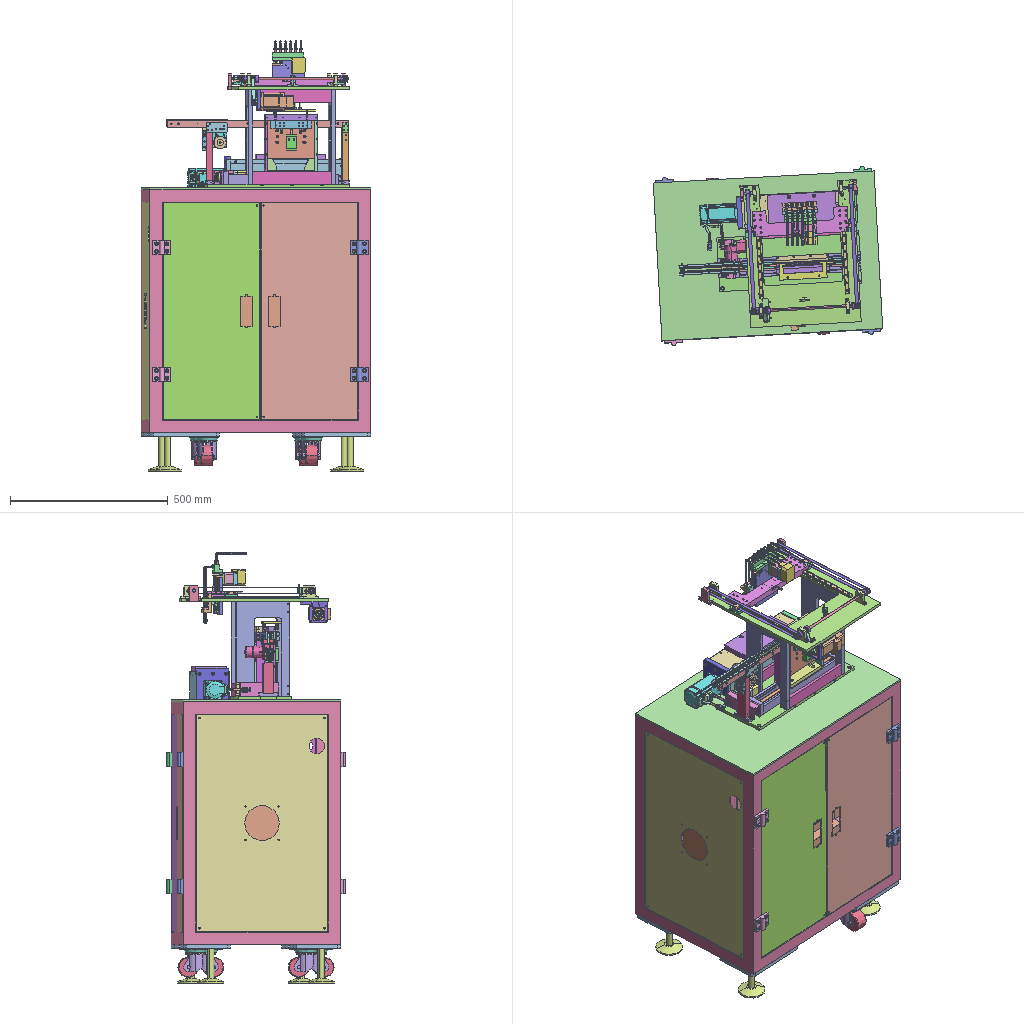Assembly | SolidWorks | 162 different items | 352 placed | box 726 x 565 x 1363 mm
Parts list (item | name | quantity | parent item | size | volume | features):
1 | (subassembly) | x2 | in 11 | 59.5 x 34.5 x 13 mm | 14643 mm3 | -
2 | (subassembly) | x1 | - | 120 x 12 x 21.25 mm | 21373 mm3 | -
3 | (subassembly) | x1 | - | 166.8 x 105 x 498.5 mm | 1079493 mm3 | -
4 | (subassembly) | x4 | in 6 | 102.5 x 91.977 x 71 mm | 201303 mm3 | -
5 | (subassembly) | x1 | - | 700 x 892 x 532 mm | 21154344 mm3 | -
6 | (subassembly) | x4 | in 5, 7 | 222 x 156.5 x 180 mm | 695134 mm3 | -
7 | (subassembly) | x2 | in 5 | 222 x 156.5 x 180 mm | 695134 mm3 | -
8 | (subassembly) | x1 | in 10 | 41 x 53 x 93.5 mm | 138509 mm3 | -
9 | (subassembly) | x1 | - | 41.5 x 52 x 94 mm | 136281 mm3 | -
10 | (subassembly) | x1 | in 11 | 131.635 x 44 x 404.935 mm | 615573 mm3 | -
11 | (subassembly) | x1 | - | 575.911 x 235.705 x 185.668 mm | 2678930 mm3 | -
12 | - | x1 | in 5 | 560 x 600 x 263 mm | 1044894 mm3 | features BaseBody 1
13 | - | x1 | - | 34 x 31 x 5 mm | 2038 mm3 | features BaseBody 1
14 | - | x2 | - | 5 x 5 x 50 mm | 981.136 mm3 | features BaseBody 1
15 | - | x1 | - | 350 x 8 x 8 mm | 17587 mm3 | features BaseBody 1
16 | - | x2 | - | 8 x 8 x 45 mm | 2262 mm3 | features BaseBody 1
17 | - | x6 | - | 10 x 10 x 77 mm | 1624 mm3 | features BaseBody 1
18 | - | x2 | in 2 | 5.001 x 5.001 x 5.2 mm | 8.924 mm3 | features BaseBody 1
19 | - | x2 | - | 17 x 23.4 x 6.7 mm | 1902 mm3 | features BaseBody 1
20 | - | x6 | - | 15 x 15 x 5 mm | 961.952 mm3 | features BaseBody 1
21 | - | x3 | - | 40 x 250 x 10 mm | 99178 mm3 | features BaseBody 1
22 | - | x1 | in 11 | 150 x 120 x 8 mm | 141574 mm3 | features BaseBody 1
23 | - | x1 | in 5 | 620 x 420 x 15 mm | 428208 mm3 | features BaseBody 1
24 | - | x1 | in 11 | 150 x 25 x 8 mm | 29604 mm3 | features BaseBody 1
25 | - | x2 | in 11 | 538 x 10 x 6 mm | 32064 mm3 | features BaseBody 1
26 | - | x1 | in 11 | 169.5 x 60 x 8 mm | 71017 mm3 | features BaseBody 1
27 | - | x1 | in 11 | 169.5 x 60 x 8 mm | 70941 mm3 | features BaseBody 1
28 | - | x2 | in 11 | 30 x 50 x 9 mm | 9481 mm3 | features BaseBody 1
29 | - | x1 | in 11 | 150 x 60 x 12 mm | 103321 mm3 | features BaseBody 1
30 | - | x1 | in 11 | 575 x 20 x 6 mm | 67891 mm3 | features BaseBody 1
31 | - | x1 | in 11 | 575 x 20 x 6 mm | 67891 mm3 | features BaseBody 1
32 | - | x2 | in 11 | 5 x 5 x 9 mm | 165.64 mm3 | features BaseBody 1
33 | - | x2 | in 2 | 3 x 3 x 16 mm | 111.003 mm3 | features BaseBody 1
34 | - | x4 | in 4 | 42 x 13 x 13 mm | 5217 mm3 | features BaseBody 1
35 | - | x2 | in 11 | 30 x 65 x 3 mm | 5483 mm3 | features BaseBody 1
36 | - | x1 | in 11 | 35 x 27 x 14.5 mm | 4375 mm3 | features BaseBody 1
37 | - | x1 | in 11 | 37 x 37 x 79.2 mm | 56499 mm3 | features BaseBody 1
38 | - | x6 | - | 10 x 10 x 13.5 mm | 457.625 mm3 | features BaseBody 1
39 | - | x1 | - | 110 x 34 x 10 mm | 36400 mm3 | features BaseBody 1
40 | - | x1 | - | 100 x 26 x 25 mm | 48829 mm3 | features BaseBody 1
41 | - | x6 | - | 8.007 x 8.002 x 20 mm | 45.848 mm3 | features BaseBody 1
42 | - | x2 | in 1 | 43 x 24 x 13 mm | 9011 mm3 | features BaseBody 1
43 | - | x2 | in 1 | 12 x 46 x 5 mm | 2467 mm3 | features BaseBody 1
44 | - | x1 | - | 16 x 11 x 16 mm | 1494 mm3 | features BaseBody 1
45 | - | x4 | in 4 | 66 x 58.3 x 58 mm | 18491 mm3 | features BaseBody 1
46 | - | x2 | - | 27 x 10 x 33.9 mm | 6982 mm3 | features BaseBody 1
47 | - | x1 | in 8 | 41 x 42.5 x 11.5 mm | 19594 mm3 | features BaseBody 1
48 | - | x1 | in 10 | 27.5 x 96.5 x 6 mm | 1654 mm3 | features BaseBody 1
49 | - | x1 | in 10 | 42.935 x 28.935 x 122.935 mm | 4950 mm3 | features BaseBody 1
50 | - | x1 | in 10 | 30 x 30 x 10.4 mm | 5208 mm3 | features BaseBody 1
51 | - | x1 | in 10 | 30 x 30 x 10.4 mm | 5208 mm3 | features BaseBody 1
52 | - | x4 | - | 48 x 40 x 10 mm | 10102 mm3 | features BaseBody 1
53 | - | x1 | in 8 | 41 x 41 x 28 mm | 43918 mm3 | features BaseBody 1
54 | - | x8 | in 11 | 12 x 12 x 19.5 mm | 1096 mm3 | features BaseBody 1
55 | - | x1 | in 9 | 41 x 41 x 29.5 mm | 16742 mm3 | features BaseBody 1
56 | - | x4 | in 4 | 58.511 x 2 x 58.511 mm | 5378 mm3 | features BaseBody 1
57 | - | x1 | in 9 | 41 x 41 x 28 mm | 45668 mm3 | features BaseBody 1
58 | - | x1 | in 9 | 41 x 41 x 11.5 mm | 19211 mm3 | features BaseBody 1
59 | - | x1 | in 9 | 41.5 x 52 x 41.5 mm | 54660 mm3 | features BaseBody 1
60 | - | x1 | in 8 | 41 x 41 x 27.5 mm | 16881 mm3 | features BaseBody 1
61 | - | x1 | in 8 | 41 x 53 x 43.5 mm | 58117 mm3 | features BaseBody 1
62 | - | x1 | - | 19.5 x 18.22 x 18.22 mm | 3669 mm3 | features BaseBody 1
63 | - | x1 | - | 8 x 8 x 5 mm | 203.222 mm3 | features BaseBody 1
64 | - | x1 | in 2 | 109 x 7 x 7 mm | 4929 mm3 | features BaseBody 1
65 | - | x12 | in 2 | 2 x 2 x 5 mm | 15.693 mm3 | features BaseBody 1
66 | - | x2 | in 10 | 45 x 18 x 46.5 mm | 29745 mm3 | features BaseBody 1
67 | - | x4 | in 4 | 96 x 14.2 x 71 mm | 54895 mm3 | features BaseBody 1
68 | - | x1 | - | 22 x 19 x 5 mm | 1962 mm3 | features BaseBody 1
69 | - | x1 | - | 700 x 500 x 6 mm | 2100000 mm3 | features Extrusion 1
70 | - | x4 | in 4 | 38 x 64.977 x 65 mm | 117327 mm3 | features BaseBody 1
71 | - | x2 | in 5 | 57.5 x 16 x 46 mm | 23419 mm3 | features BaseBody 1
72 | - | x4 | in 6 | 85 x 180 x 85 mm | 108156 mm3 | features BaseBody 1
73 | - | x4 | in 5 | 57.5 x 16 x 46 mm | 23419 mm3 | features BaseBody 1
74 | - | x2 | - | 7 x 4.7 x 40 mm | 1153 mm3 | features BaseBody 1
75 | - | x2 | in 5 | 57.5 x 16 x 46 mm | 23419 mm3 | features BaseBody 1
76 | - | x1 | in 3 | 335 x 15 x 15 mm | 55455 mm3 | features BaseBody 1
77 | - | x1 | in 3 | 52 x 57 x 34 mm | 42280 mm3 | features BaseBody 1
78 | - | x2 | in 3 | 15 x 10 x 283 mm | 39191 mm3 | features BaseBody 1
79 | - | x4 | in 3 | 32 x 12 x 58.8 mm | 16967 mm3 | features BaseBody 5
80 | - | x1 | in 3 | 44 x 46 x 46 mm | 54630 mm3 | features BaseBody 1
81 | - | x1 | in 3 | 98 x 102 x 15 mm | 114752 mm3 | features BaseBody 1
82 | - | x1 | in 3 | 102 x 12 x 353 mm | 381378 mm3 | features BaseBody 1
83 | - | x1 | in 3 | 216 x 100 x 17 mm | 362258 mm3 | features HoleWzd 2, Extrusion 1
84 | - | x1 | in 3 | 15 x 75 x 102 mm | 56367 mm3 | features BaseBody 1
85 | - | x1 | - | 32 x 12 x 42.4 mm | 12424 mm3 | features BaseBody 1
86 | - | x1 | in 3 | 102 x 12 x 71.5 mm | 59210 mm3 | features BaseBody 1
87 | - | x1 | in 3 | 70 x 40 x 40 mm | 71369 mm3 | features BaseBody 1
88 | - | x1 | in 3 | 380 x 104 x 88 mm | 108125 mm3 | features BaseBody 1
89 | - | x2 | in 3 | 8 x 26 x 26 mm | 2684 mm3 | features BaseBody 1
90 | - | x2 | in 3 | 31 x 10 x 10 mm | 1099 mm3 | features BaseBody 1
91 | - | x1 | in 3 | - | - | features RefSurface 7
92 | - | x1 | in 5 | 308 x 688 x 15 mm | 352674 mm3 | features BaseBody 1
93 | - | x2 | in 5 | 308 x 688 x 15 mm | 352674 mm3 | features BaseBody 1
94 | - | x6 | - | 6 x 19 x 19 mm | 1232 mm3 | features BaseBody 1
95 | - | x1 | in 10 | 122 x 43.5 x 6 mm | 22091 mm3 | features BaseBody 1
96 | - | x1 | in 5 | 700 x 770 x 500 mm | 13960000 mm3 | features BaseBody 1
97 | - | x1 | in 10 | 60.2 x 43.4 x 392 mm | 378464 mm3 | features BaseBody 2
98 | - | x1 | in 11 | 51 x 24 x 14 mm | 14438 mm3 | features BaseBody 1
99 | - | x1 | in 11 | 5 x 5 x 50 mm | 907.789 mm3 | features BaseBody 1
100 | - | x1 | in 11 | 6.928 x 8 x 2.4 mm | 78.962 mm3 | features BaseBody 1
101 | - | x1 | - | 29 x 51 x 13.5 mm | 18511 mm3 | features BaseBody 1
102 | - | x2 | - | 48 x 50 x 10 mm | 13107 mm3 | features BaseBody 1
103 | - | x1 | - | 8 x 20 x 14 mm | 1764 mm3 | features BaseBody 1
104 | - | x1 | - | 8 x 14 x 6 mm | 556.546 mm3 | features BaseBody 1
105 | - | x2 | - | 40 x 18 x 25 mm | 10257 mm3 | features BaseBody 1
106 | - | x2 | - | 13 x 25 x 9 mm | 2752 mm3 | features BaseBody 1
107 | - | x16 | in 5 | 60 x 60 x 30 mm | 28435 mm3 | features BaseBody 1
108 | - | x2 | - | 395.01 x 21.01 x 10 mm | 8109 mm3 | features BaseBody 1
109 | - | x12 | - | 11 x 5 x 5.774 mm | 106.233 mm3 | features BaseBody 1
110 | - | x1 | - | 85 x 66 x 8 mm | 18162 mm3 | features BaseBody 1
111 | - | x1 | in 11 | 40 x 40 x 23 mm | 24363 mm3 | features BaseBody 1
112 | - | x1 | in 2 | 120 x 12 x 15 mm | 9058 mm3 | features BaseBody 1
113 | - | x1 | in 2 | 120 x 12 x 5 mm | 6743 mm3 | features BaseBody 1
114 | - | x12 | in 2 | 3.2 x 2.4 x 1.65 mm | 5.798 mm3 | features BaseBody 1
115 | - | x1 | - | 56 x 126.1 x 70.6 mm | 288877 mm3 | features BaseBody 1
116 | - | x1 | - | 5 x 5 x 41 mm | 724.909 mm3 | features BaseBody 1
117 | - | x1 | in 11 | 12 x 12 x 9 mm | 755.086 mm3 | features BaseBody 1
118 | - | x4 | in 6 | 220 x 150 x 12 mm | 385674 mm3 | features BaseBody 1
119 | - | x1 | in 11 | 24 x 50 x 11.5 mm | 13579 mm3 | features BaseBody 1
120 | - | x2 | in 11 | 85 x 569 x 5 mm | 6467 mm3 | features BaseBody 1
121 | - | x1 | in 11 | 65 x 50 x 4 mm | 11503 mm3 | features BaseBody 1
122 | - | x1 | - | 110 x 60 x 25 mm | 92484 mm3 | features BaseBody 1
123 | - | x12 | - | 4 x 95.26 x 25.9 mm | 632.21 mm3 | features BaseBody 1
124 | - | x1 | - | 98.817 x 21.817 x 10 mm | 2968 mm3 | features BaseBody 1
125 | - | x2 | - | 22 x 22 x 15 mm | 3752 mm3 | features BaseBody 1
126 | - | x1 | - | 23 x 22 x 22 mm | 6448 mm3 | features BaseBody 1
127 | - | x3 | - | 23 x 22 x 22 mm | 5708 mm3 | features BaseBody 1
128 | - | x2 | in 11 | 190 x 9 x 5 mm | 6549 mm3 | features BaseBody 1
129 | - | x1 | in 5 | 418 x 688 x 15 mm | 443799 mm3 | features BaseBody 1
130 | - | x1 | in 11 | 166 x 23 x 19 mm | 61656 mm3 | features BaseBody 1
131 | - | x1 | in 11 | 166 x 30 x 19 mm | 83734 mm3 | features BaseBody 1
132 | - | x1 | in 11 | 37 x 35 x 17 mm | 3884 mm3 | features BaseBody 1
133 | - | x1 | in 11 | 42 x 20 x 3 mm | 2109 mm3 | features BaseBody 1
134 | - | x1 | in 11 | 120 x 50 x 20 mm | 67533 mm3 | features BaseBody 1
135 | - | x2 | in 1 | 12 x 19 x 5 mm | 849.461 mm3 | features BaseBody 1
136 | - | x2 | in 1 | 5 x 44 x 3.7 mm | 746.693 mm3 | features BaseBody 1
137 | - | x2 | in 11 | 30 x 20 x 8 mm | 3357 mm3 | features BaseBody 1
138 | - | x2 | in 11 | 54 x 9 x 6 mm | 2740 mm3 | features BaseBody 1
139 | - | x1 | - | 130 x 25 x 10 mm | 22368 mm3 | features BaseBody 1
140 | - | x1 | in 5 | 418 x 688 x 15 mm | 443799 mm3 | features BaseBody 1
141 | - | x1 | - | 150 x 52.5 x 5 mm | 19392 mm3 | features BaseBody 1
142 | - | x12 | - | 9 x 11.899 x 12 mm | 248.45 mm3 | features BaseBody 1
143 | - | x1 | - | 100 x 135 x 10 mm | 119141 mm3 | features BaseBody 1
144 | - | x2 | - | 2.5 x 2.5 x 15 mm | 72.605 mm3 | features BaseBody 1
145 | - | x1 | in 11 | 450 x 170 x 10 mm | 751937 mm3 | features BaseBody 1
146 | - | x2 | in 2 | 7 x 7 x 5.8 mm | 72.379 mm3 | features BaseBody 1
147 | - | x1 | - | 80 x 302 x 20 mm | 261763 mm3 | features BaseBody 1
148 | - | x6 | - | 8 x 8 x 15 mm | 358.289 mm3 | features BaseBody 1
149 | - | x2 | - | 300 x 170 x 12 mm | 349204 mm3 | features BaseBody 1
150 | - | x2 | - | 26 x 13.5 x 6 mm | 1123 mm3 | features BaseBody 1
151 | - | x1 | in 5 | 308 x 688 x 15 mm | 352604 mm3 | features BaseBody 1
152 | - | x2 | in 1 | 3 x 3 x 20 mm | 140.324 mm3 | features BaseBody 1
153 | - | x2 | in 1 | 32 x 12 x 5 mm | 1429 mm3 | features BaseBody 1
154 | - | x2 | in 11 | 20 x 30 x 3 mm | 1654 mm3 | features BaseBody 1
155 | - | x1 | in 11 | 173.5 x 33 x 20 mm | 108000 mm3 | features BaseBody 1
156 | - | x2 | in 11 | 20 x 60 x 12 mm | 9580 mm3 | features BaseBody 1
157 | - | x1 | in 11 | 173.5 x 33 x 20 mm | 112617 mm3 | features BaseBody 1
158 | - | x1 | - | 14.22 x 116.22 x 6 mm | 1473 mm3 | features BaseBody 1
159 | - | x2 | - | 12 x 7.5 x 270 mm | 21191 mm3 | features BaseBody 1
160 | - | x1 | - | 450 x 350 x 10 mm | 754366 mm3 | features BaseBody 1
161 | - | x2 | - | 23.5 x 6 x 24 mm | 787.031 mm3 | features BaseBody 1
162 | - | x1 | - | 15 x 9.5 x 110 mm | 14193 mm3 | features BaseBody 1
Mates (type | each side: item.copy, entity, surface, feature):
In the top assembly
Parallel | 149.1 face plane input1 | 160.1 face plane input1
Coincident | 149.1 face plane input1 | 160.1 face plane input1
Concentric | 160.1 face cylinder input1 | 159.1 face cylinder input1
Coincident | 69.1 face plane Boss-Extrude1 | 96.1 face plane input1 | 3 times
Coincident | 145.1 face plane input1 | 69.1 face plane Boss-Extrude1
Width | 96.1 face plane input1 | 96.1 face plane input1 | 30.1 face plane input1 | 160.1 face plane input1
DistanceDim | 160.1 face plane input1 | 96.1 face plane input1
Coincident | 69.1 face plane Boss-Extrude1 | 88.1 face plane input1
Parallel | 96.1 face plane input1 | 88.1 face plane input1
In subassembly 3
Coincident | 82.1 face plane input1 | 83.1 face plane Boss-Extrude1
Width | 83.1 face plane Boss-Extrude1 | 83.1 face plane Boss-Extrude1 | 88.2 face plane input1 | 88.2 face plane input1